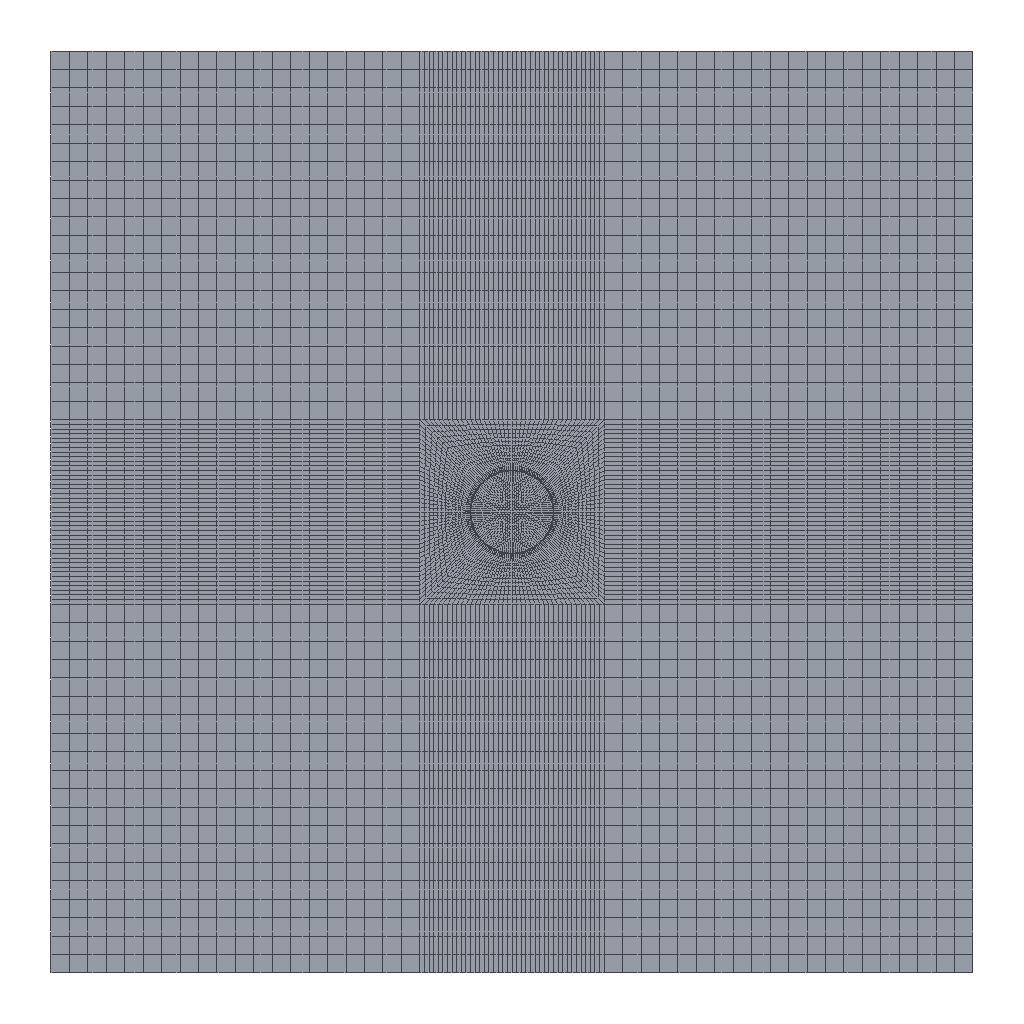Simulation study | abaqus
Set-up summary:
category,name,step,type,value,unit,region
solver,abaqus,,Abaqus/CAE 2024
units,SI m-kg-s (Pa),,inferred,E=2e+10 density=2500
analysis,Step-Geostatic,,geostatic,nlgeom=True; time_period=1
analysis,Step-Excavation,,static,nlgeom=True; time_period=1
analysis,Step-Support,,static,nlgeom=True; time_period=1
analysis,Step-Pressure,,static,nlgeom=True; time_period=8
mesh,nodes,,,10837
mesh,elements,,,10120
element_type,CPE4R,,,8911
element_type,CPE4RH,,,1209
material,Rock,,E,2e+10
material,Rock,,nu,0.25
material,Rock,,density,2500
material,Rubber,,behaviors,hyperelastic
material,UHPC,,E,4.5e+10
material,UHPC,,nu,0.2
material,UHPC,,density,2500
material,UHPC,,behaviors,plastic; concrete damaged plasticity; concrete compression hardening; concrete tension stiffening; concrete compression damage; concrete tension damage
section,Rock,,solid section,,,_PickedSet80
section,Rubber,,solid section,,,_PickedSet2
section,UHPC,,solid section,,,_PickedSet5
load,Load-1,Step-Geostatic,gravity,9.81,,whole model
load,Load-2,Step-Geostatic,pressure,1e+07,,_PickedSurf7
load,Load-3,Step-Geostatic,pressure,1.25e+07,,_PickedSurf8
load,Gas,Step-Pressure,pressure,5e+06,,"Rubber-1.""Rubber inside"""
bc,Bottom,initial,fixed,[dofs=y],,_PickedSet6
bc,Left,initial,fixed,[dofs=x],,_PickedSet4
bc,Right,initial,fixed,[dofs=x],,_PickedSet5
contact,UHPC Rock,initial,tie,,,"UHPC-1.""UHPC outside"" / Cavern-Geostress-1.""Rock inside"""
contact,Int-8,initial,contact pair surface to surface,interaction=Basic 1; friction=0.3; behavior=hard,,"Rubber-1.""Rubber outside"" / UHPC-1.""UHPC inside"""
Abaqus input file, long lists of numbers shortened:
*Heading
** Job name: deck Model name: Model-2
** Generated by: Abaqus/CAE 2024
*Preprint, echo=NO, model=NO, history=NO, contact=NO
**
** PARTS
**
*Part, name=Cavern-Geostress
*Node
      1,         -10.,          10.
      2,         -10.,          50.
** (7999 more lines like these left out)
*Element, type=CPE4R
  1,    1,   30,  970,  105
  2,   30,   31,  971,  970
** (7838 more lines like these left out)
*Nset, nset=_PickedSet80, internal, generate
    1,  8001,     1
*Elset, elset=_PickedSet80, internal, generate
    1,  7840,     1
*Elset, elset="_Rock inside_S2", internal
 2101, 2102, 2103, 2104, 2105, 2106, 2107, 2108, 2109, 2110, 2221, 2222, 2223, 2224, 2225, 2226
 2227, 2228, 2229, 2230, 2341, 2342, 2343, 2344, 2345, 2346, 2347, 2348, 2349, 2350, 2981, 2982
** (3 more lines like these left out)
*Elset, elset="_Rock inside_S1", internal
 2111, 2112, 2113, 2114, 2115, 2116, 2117, 2118, 2119, 2120, 2231, 2232, 2233, 2234, 2235, 2236
 2237, 2238, 2239, 2240, 2351, 2352, 2353, 2354, 2355, 2356, 2357, 2358, 2359, 2360, 2991, 2992
** (3 more lines like these left out)
*Surface, type=ELEMENT, name="Rock inside"
"_Rock inside_S2", S2
"_Rock inside_S1", S1
** Section: Section-1
*Solid Section, elset=_PickedSet80, material=Rock
,
*End Part
**
*Part, name=Rubber
*Node
      1, 0.002345,  -4.5
      2, 0.002345,  -4.46
** (1610 more lines like these left out)
*Element, type=CPE4RH
  1,   1,  18, 823, 121
  2,  18,  19, 824, 823
** (1207 more lines like these left out)
*Nset, nset=_PickedSet2, internal, generate
    1,  1612,     1
*Elset, elset=_PickedSet2, internal, generate
    1,  1209,     1
*Nset, nset="Edge Seeds-Rubber"
   1,   2,   3,   4,   5,   6,   7,   8,   9,  10,  12,  13,  14,  15,  16,  17
  18,  19,  70,  71, 171, 172, 222, 223, 322, 323, 473, 474, 574, 575, 625, 626
*Elset, elset="Edge Seeds-Rubber"
    1,    2,    3,  151,  152,  153,  154,  155,  156,  301,  302,  303,  304,  305,  306,  451
  452,  453,  454,  455,  456,  604,  605,  606,  607,  608,  609,  757,  758,  759,  760,  761
** (1 more lines like these left out)
*Elset, elset="_Rubber outside_S4", internal
    1,    4,    7,   10,   13,   16,   19,   22,   25,   28,   31,   34,   37,   40,   43,   46
   49,   52,   55,   58,   61,   64,   67,   70,   73,   76,   79,   82,   85,   88,   91,   94
** (11 more lines like these left out)
*Elset, elset="_Rubber outside_S2", internal
  156,  159,  162,  165,  168,  171,  174,  177,  180,  183,  186,  189,  192,  195,  198,  201
  204,  207,  210,  213,  216,  219,  222,  225,  228,  231,  234,  237,  240,  243,  246,  249
** (11 more lines like these left out)
*Surface, type=ELEMENT, name="Rubber outside"
"_Rubber outside_S4", S4
"_Rubber outside_S2", S2
*Elset, elset="_Rubber inside_S2", internal
    3,    6,    9,   12,   15,   18,   21,   24,   27,   30,   33,   36,   39,   42,   45,   48
   51,   54,   57,   60,   63,   66,   69,   72,   75,   78,   81,   84,   87,   90,   93,   96
** (11 more lines like these left out)
*Elset, elset="_Rubber inside_S4", internal
  154,  157,  160,  163,  166,  169,  172,  175,  178,  181,  184,  187,  190,  193,  196,  199
  202,  205,  208,  211,  214,  217,  220,  223,  226,  229,  232,  235,  238,  241,  244,  247
** (11 more lines like these left out)
*Surface, type=ELEMENT, name="Rubber inside"
"_Rubber inside_S2", S2
"_Rubber inside_S4", S4
** Section: Section-3
*Solid Section, elset=_PickedSet2, material=Rubber
,
*End Part
**
*Part, name=UHPC
*Node
      1,  -3.536,  -3.536
      2,  -3.182,  -3.182
** (1222 more lines like these left out)
*Element, type=CPE4R
  1,   1,  19, 355,  66
  2,  19,  20, 356, 355
** (1069 more lines like these left out)
*Nset, nset=_PickedSet5, internal, generate
    1,  1224,     1
*Elset, elset=_PickedSet5, internal, generate
    1,  1071,     1
*Elset, elset="_UHPC outside_S4", internal
    1,    8,   15,   22,   29,   36,   43,   50,   57,   64,   71,   78,   85,   92,   99,  106
  113,  120,  127,  400,  407,  414,  421,  428,  435,  442,  449,  456,  463,  470,  477,  484
** (3 more lines like these left out)
*Elset, elset="_UHPC outside_S2", internal
 140, 147, 154, 161, 168, 175, 182, 189, 196, 203, 210, 217, 224, 231, 238, 245
 252, 259, 266, 273, 280, 287, 294, 301, 308, 315, 322, 329, 336, 343, 350, 357
** (3 more lines like these left out)
*Surface, type=ELEMENT, name="UHPC outside"
"_UHPC outside_S4", S4
"_UHPC outside_S2", S2
*Elset, elset="_UHPC inside_S2", internal
    7,   14,   21,   28,   35,   42,   49,   56,   63,   70,   77,   84,   91,   98,  105,  112
  119,  126,  133,  406,  413,  420,  427,  434,  441,  448,  455,  462,  469,  476,  483,  490
** (3 more lines like these left out)
*Elset, elset="_UHPC inside_S4", internal
 134, 141, 148, 155, 162, 169, 176, 183, 190, 197, 204, 211, 218, 225, 232, 239
 246, 253, 260, 267, 274, 281, 288, 295, 302, 309, 316, 323, 330, 337, 344, 351
** (3 more lines like these left out)
*Surface, type=ELEMENT, name="UHPC inside"
"_UHPC inside_S2", S2
"_UHPC inside_S4", S4
** Section: Section-2
*Solid Section, elset=_PickedSet5, material=UHPC
,
*End Part
**
**
** ASSEMBLY
**
*Assembly, name=Assembly
**
*Instance, name=Cavern-Geostress-1, part=Cavern-Geostress
*End Instance
**
*Instance, name=Rubber-1, part=Rubber
*End Instance
**
*Instance, name=UHPC-1, part=UHPC
          0.,           0.,           0.
          0.,           0.,           0.,           0.,           0., 1., 90.
*End Instance
**
*Nset, nset=_PickedSet4, internal, instance=Cavern-Geostress-1
   3,   4,  10,  11,  68,  69,  70,  71,  72,  73,  74,  75,  76,  77,  78,  79
  80,  81,  82,  83,  84,  85,  86, 240, 241, 242, 243, 244, 245, 246, 247, 248
** (4 more lines like these left out)
*Elset, elset=_PickedSet4, internal, instance=Cavern-Geostress-1
  381,  382,  383,  384,  385,  386,  387,  388,  389,  390,  391,  392,  393,  394,  395,  396
  397,  398,  399,  400, 1581, 1582, 1583, 1584, 1585, 1586, 1587, 1588, 1589, 1590, 1591, 1592
** (3 more lines like these left out)
*Nset, nset=_PickedSet5, internal, instance=Cavern-Geostress-1
  14,  15,  25,  29, 316, 317, 318, 319, 320, 321, 322, 323, 324, 325, 326, 327
 328, 329, 330, 331, 332, 333, 334, 653, 654, 655, 656, 657, 658, 659, 660, 661
** (4 more lines like these left out)
*Elset, elset=_PickedSet5, internal, instance=Cavern-Geostress-1
 1981, 1982, 1983, 1984, 1985, 1986, 1987, 1988, 1989, 1990, 1991, 1992, 1993, 1994, 1995, 1996
 1997, 1998, 1999, 2000, 4200, 4220, 4240, 4260, 4280, 4300, 4320, 4340, 4360, 4380, 4400, 4420
** (3 more lines like these left out)
*Nset, nset=_PickedSet6, internal, instance=Cavern-Geostress-1
   8,  11,  13,  14, 259, 260, 261, 262, 263, 264, 265, 266, 267, 268, 269, 270
 271, 272, 273, 274, 275, 276, 277, 297, 298, 299, 300, 301, 302, 303, 304, 305
** (4 more lines like these left out)
*Elset, elset=_PickedSet6, internal, instance=Cavern-Geostress-1
 1201, 1221, 1241, 1261, 1281, 1301, 1321, 1341, 1361, 1381, 1401, 1421, 1441, 1461, 1481, 1501
 1521, 1541, 1561, 1581, 1620, 1640, 1660, 1680, 1700, 1720, 1740, 1760, 1780, 1800, 1820, 1840
** (3 more lines like these left out)
*Nset, nset=_PickedSet10, internal, instance=Cavern-Geostress-1
   16,   17,   18,   19,   20,   23,   24,   26,   27,  354,  355,  356,  357,  358,  359,  360
  361,  362,  363,  364,  365,  366,  367,  368,  369,  370,  371,  372,  373,  374,  375,  376
** (64 more lines like these left out)
*Elset, elset=_PickedSet10, internal, instance=Cavern-Geostress-1
 2001, 2002, 2003, 2004, 2005, 2006, 2007, 2008, 2009, 2010, 2011, 2012, 2013, 2014, 2015, 2016
 2017, 2018, 2019, 2020, 2021, 2022, 2023, 2024, 2025, 2026, 2027, 2028, 2029, 2030, 2031, 2032
** (58 more lines like these left out)
*Nset, nset=_PickedSet32, internal, instance=UHPC-1, generate
    1,  1224,     1
*Elset, elset=_PickedSet32, internal, instance=UHPC-1, generate
    1,  1071,     1
*Nset, nset=_PickedSet33, internal, instance=UHPC-1, generate
    1,  1224,     1
*Elset, elset=_PickedSet33, internal, instance=UHPC-1, generate
    1,  1071,     1
*Nset, nset=_PickedSet34, internal, instance=Rubber-1, generate
    1,  1612,     1
*Elset, elset=_PickedSet34, internal, instance=Rubber-1, generate
    1,  1209,     1
*Nset, nset=_PickedSet35, internal, instance=Rubber-1, generate
    1,  1612,     1
*Elset, elset=_PickedSet35, internal, instance=Rubber-1, generate
    1,  1209,     1
*Elset, elset=__PickedSurf7_S3, internal, instance=Cavern-Geostress-1
  381,  382,  383,  384,  385,  386,  387,  388,  389,  390,  391,  392,  393,  394,  395,  396
  397,  398,  399,  400, 1581, 1582, 1583, 1584, 1585, 1586, 1587, 1588, 1589, 1590, 1591, 1592
** (3 more lines like these left out)
*Elset, elset=__PickedSurf7_S4, internal, instance=Cavern-Geostress-1, generate
 5741,  6521,    20
*Elset, elset=__PickedSurf7_S2, internal, instance=Cavern-Geostress-1, generate
 4200,  4980,    20
*Surface, type=ELEMENT, name=_PickedSurf7, internal
__PickedSurf7_S3, S3
__PickedSurf7_S4, S4
__PickedSurf7_S2, S2
*Elset, elset=__PickedSurf8_S2, internal, instance=Cavern-Geostress-1, generate
   20,  1200,    20
*Elset, elset=__PickedSurf8_S4, internal, instance=Cavern-Geostress-1, generate
 6541,  6921,    20
*Surface, type=ELEMENT, name=_PickedSurf8, internal
__PickedSurf8_S2, S2
__PickedSurf8_S4, S4
** Constraint: UHPC Rock
*Tie, name="UHPC Rock", adjust=yes
UHPC-1."UHPC outside", Cavern-Geostress-1."Rock inside"
*End Assembly
*Amplitude, name=Cycle
             0.,              0.,             0.1,             0.5,             0.2,              1.,              2.,              1.
             3.,             0.8,              4.,             0.5,              5.,             0.2,              6.,              0.
             8.,              0.
**
** MATERIALS
**
*Material, name=Rock
*Density
2500.,
*Elastic
 2e+10, 0.25
*Material, name=Rubber
*Hyperelastic, mooney-rivlin
400000.,100000.,   0.01
*Material, name=UHPC
*Density
2500.,
*Elastic
 4.5e+10, 0.2
*Concrete Damaged Plasticity
30.,    0.1,   1.16, 0.6667,   0.05
*Concrete Compression Hardening
    6e+07,      0.
    7e+07,   5e-05
    8e+07, 0.00012
    9e+07, 0.00022
    1e+08, 0.00036
 1.08e+08, 0.00055
 1.14e+08, 0.00078
 1.19e+08, 0.00105
 1.23e+08, 0.00135
 1.26e+08,  0.0017
 1.25e+08, 0.00205
 1.23e+08, 0.00245
 1.21e+08,  0.0029
 1.18e+08,  0.0034
 1.15e+08,   0.004
 1.11e+08,  0.0047
 1.07e+08,  0.0056
 1.02e+08,  0.0067
  9.6e+07,   0.008
    9e+07,  0.0095
  8.2e+07,  0.0115
  7.4e+07,   0.014
  6.6e+07,   0.017
  5.8e+07,    0.02
*Concrete Tension Stiffening
    1e+07,      0.
 1.15e+07,   2e-05
 1.25e+07,   5e-05
  1.2e+07,  0.0001
  1.1e+07,  0.0002
    1e+07, 0.00035
  8.8e+06, 0.00055
  7.5e+06,  0.0008
  6.2e+06,  0.0012
    5e+06,  0.0018
  3.8e+06,  0.0026
  2.8e+06,  0.0037
    2e+06,  0.0052
  1.2e+06,   0.007
  500000.,    0.01
*Concrete Compression Damage
    0.,      0.
 0.002,   5e-05
 0.005, 0.00012
  0.01, 0.00022
 0.018, 0.00036
  0.03, 0.00055
 0.045, 0.00078
 0.065, 0.00105
  0.09, 0.00135
  0.12,  0.0017
  0.16, 0.00205
  0.21, 0.00245
  0.27,  0.0029
  0.34,  0.0034
  0.42,   0.004
   0.5,  0.0047
  0.58,  0.0056
   0.6,  0.0067
  0.62,   0.008
  0.64,  0.0095
  0.66,  0.0115
  0.68,   0.014
   0.7,   0.017
  0.72,    0.02
*Concrete Tension Damage
   0.,      0.
 0.01,   2e-05
 0.03,   5e-05
 0.06,  0.0001
  0.1,  0.0002
 0.16, 0.00035
 0.24, 0.00055
 0.34,  0.0008
 0.46,  0.0012
 0.58,  0.0018
  0.7,  0.0026
  0.8,  0.0037
 0.88,  0.0052
 0.94,   0.007
 0.99,    0.01
**
** INTERACTION PROPERTIES
**
*Surface Interaction, name="Basic 1"
1.,
*Friction, slip tolerance=0.005
 0.3,
*Surface Behavior, pressure-overclosure=HARD
*Surface Interaction, name="Basic 2"
1.,
*Friction, slip tolerance=0.005
 0.4,
*Surface Behavior, pressure-overclosure=HARD
**
** BOUNDARY CONDITIONS
**
** Name: Bottom bd Type: Displacement/Rotation
*Boundary
_PickedSet6, 2, 2
** Name: Left bd Type: Displacement/Rotation
*Boundary
_PickedSet4, 1, 1
** Name: Right bd Type: Displacement/Rotation
*Boundary
_PickedSet5, 1, 1
**
** INTERACTIONS
**
** Interaction: Int-8
*Contact Pair, interaction="Basic 1", type=SURFACE TO SURFACE
Rubber-1."Rubber outside", UHPC-1."UHPC inside"
** ----------------------------------------------------------------
**
** STEP: Step-Geostatic
**
*Step, name=Step-Geostatic, nlgeom=YES
*Geostatic, utol
0.1, 1., 1e-05, 1.
**
** LOADS
**
** Name: Load-1   Type: Gravity
*Dload
, GRAV, 9.81, 0., -1.
** Name: Load-2   Type: Pressure
*Dsload
_PickedSurf7, P, 1e+07
** Name: Load-3   Type: Pressure
*Dsload
_PickedSurf8, P, 1.25e+07
**
** INTERACTIONS
**
** Interaction: Delete Rubber
*Model Change, remove
_PickedSet34,
** Interaction: Delete UHPC
*Model Change, remove
_PickedSet33,
** Interaction: Int-8
*Model Change, type=CONTACT PAIR, remove
Rubber-1."Rubber outside", UHPC-1."UHPC inside"
**
** OUTPUT REQUESTS
**
*Restart, write, frequency=0
**
** FIELD OUTPUT: F-Output-1
**
*Output, field, variable=PRESELECT
**
** HISTORY OUTPUT: H-Output-1
**
*Output, history, variable=PRESELECT
*End Step
** ----------------------------------------------------------------
**
** STEP: Step-Excavation
**
*Step, name=Step-Excavation, nlgeom=YES, inc=500
*Static, stabilize=0.0002, allsdtol=0.05, continue=NO
0.02, 1., 1e-06, 0.1
**
** INTERACTIONS
**
** Interaction: Delete Rubber
*Model Change, add
_PickedSet34,
** Interaction: Delete UHPC
*Model Change, add
_PickedSet33,
** Interaction: Excavation
*Model Change, remove
_PickedSet10,
** Interaction: Int-8
*Model Change, type=CONTACT PAIR, add
Rubber-1."Rubber outside", UHPC-1."UHPC inside"
**
** OUTPUT REQUESTS
**
*Restart, write, frequency=0
**
** FIELD OUTPUT: F-Output-1
**
*Output, field, variable=PRESELECT
**
** HISTORY OUTPUT: H-Output-1
**
*Output, history, variable=PRESELECT
*End Step
** ----------------------------------------------------------------
**
** STEP: Step-Support
**
*Step, name=Step-Support, nlgeom=YES
Add UHPC Rubber
*Static, stabilize=0.0002, allsdtol=0.05, continue=NO
0.01, 1., 1e-10, 0.1
**
** OUTPUT REQUESTS
**
*Restart, write, frequency=0
**
** FIELD OUTPUT: F-Output-1
**
*Output, field
*Node Output
CF, RF, U
*Element Output, directions=YES
DAMAGEC, DAMAGET, LE, PE, PEEQ, PEMAG, S
*Contact Output
CDISP, CSTRESS
**
** HISTORY OUTPUT: H-Output-1
**
*Output, history, variable=PRESELECT
*End Step
** ----------------------------------------------------------------
**
** STEP: Step-Pressure
**
*Step, name=Step-Pressure, nlgeom=YES, inc=1000
*Static, stabilize=0.0002, allsdtol=0.05, continue=NO
0.001, 8., 1e-10, 0.01
**
** LOADS
**
** Name: Gas Pressure   Type: Pressure
*Dsload, amplitude=Cycle
Rubber-1."Rubber inside", P, 5e+06
**
** OUTPUT REQUESTS
**
*Restart, write, frequency=0
**
** FIELD OUTPUT: F-Output-1
**
*Output, field
*Node Output
CF, RF, U
*Element Output, directions=YES
DAMAGEC, DAMAGET, LE, PE, PEEQ, PEMAG, S
*Contact Output
CDISP, CSTRESS
**
** HISTORY OUTPUT: H-Output-1
**
*Output, history, variable=PRESELECT
*End Step
Results summary:
result,odb.job_status,,,JOB_STATUS_COMPLETED_SUCCESSFULLY,"consistent, unstated (Abaqus has no unit system)"
result,steps[0].procedure,Step-Geostatic,,*GEOSTATIC,"consistent, unstated (Abaqus has no unit system)"
result,steps[0].time_period,Step-Geostatic,,1,"consistent, unstated (Abaqus has no unit system)"
result,steps[0].n_frames,Step-Geostatic,,7,"consistent, unstated (Abaqus has no unit system)"
result,steps[0].last_frame.id,Step-Geostatic,,6,"consistent, unstated (Abaqus has no unit system)"
result,steps[0].last_frame.value,Step-Geostatic,,1,"consistent, unstated (Abaqus has no unit system)"
result,steps[0].last_frame.description,Step-Geostatic,,Increment      6: Step Time =    1.000,"consistent, unstated (Abaqus has no unit system)"
result,steps[0].completed,Step-Geostatic,,True,"consistent, unstated (Abaqus has no unit system)"
result,steps[0].max_U_magnitude,Step-Geostatic,,1.25548e-07,"consistent, unstated (Abaqus has no unit system)"
result,steps[0].max_S_mises,Step-Geostatic,,9.95198e+06,"consistent, unstated (Abaqus has no unit system)"
result,steps[0].RF_sum[1],Step-Geostatic,,26,"consistent, unstated (Abaqus has no unit system)"
result,steps[0].RF_sum[2],Step-Geostatic,,1.49525e+09,"consistent, unstated (Abaqus has no unit system)"
result,steps[1].procedure,Step-Excavation,,*STATIC,"consistent, unstated (Abaqus has no unit system)"
result,steps[1].time_period,Step-Excavation,,1,"consistent, unstated (Abaqus has no unit system)"
result,steps[1].n_frames,Step-Excavation,,15,"consistent, unstated (Abaqus has no unit system)"
result,steps[1].last_frame.id,Step-Excavation,,14,"consistent, unstated (Abaqus has no unit system)"
result,steps[1].last_frame.value,Step-Excavation,,1,"consistent, unstated (Abaqus has no unit system)"
result,steps[1].last_frame.description,Step-Excavation,,Increment     14: Step Time =    1.000,"consistent, unstated (Abaqus has no unit system)"
result,steps[1].completed,Step-Excavation,,True,"consistent, unstated (Abaqus has no unit system)"
result,steps[1].max_U_magnitude,Step-Excavation,,0.00606,"consistent, unstated (Abaqus has no unit system)"
result,steps[1].max_S_mises,Step-Excavation,,4.03912e+07,"consistent, unstated (Abaqus has no unit system)"
result,steps[1].RF_sum[1],Step-Excavation,,77,"consistent, unstated (Abaqus has no unit system)"
result,steps[1].RF_sum[2],Step-Excavation,,1.49367e+09,"consistent, unstated (Abaqus has no unit system)"
result,steps[2].procedure,Step-Support,,*STATIC,"consistent, unstated (Abaqus has no unit system)"
result,steps[2].time_period,Step-Support,,1,"consistent, unstated (Abaqus has no unit system)"
result,steps[2].n_frames,Step-Support,,16,"consistent, unstated (Abaqus has no unit system)"
result,steps[2].last_frame.id,Step-Support,,15,"consistent, unstated (Abaqus has no unit system)"
result,steps[2].last_frame.value,Step-Support,,1,"consistent, unstated (Abaqus has no unit system)"
result,steps[2].last_frame.description,Step-Support,,Increment     15: Step Time =    1.000,"consistent, unstated (Abaqus has no unit system)"
result,steps[2].completed,Step-Support,,True,"consistent, unstated (Abaqus has no unit system)"
result,steps[2].max_U_magnitude,Step-Support,,0.006061,"consistent, unstated (Abaqus has no unit system)"
result,steps[2].max_S_mises,Step-Support,,4.03922e+07,"consistent, unstated (Abaqus has no unit system)"
result,steps[2].RF_sum[1],Step-Support,,87,"consistent, unstated (Abaqus has no unit system)"
result,steps[2].RF_sum[2],Step-Support,,1.49369e+09,"consistent, unstated (Abaqus has no unit system)"
result,steps[3].procedure,Step-Pressure,,*STATIC,"consistent, unstated (Abaqus has no unit system)"
result,steps[3].time_period,Step-Pressure,,8,"consistent, unstated (Abaqus has no unit system)"
result,steps[3].n_frames,Step-Pressure,,810,"consistent, unstated (Abaqus has no unit system)"
result,steps[3].last_frame.id,Step-Pressure,,809,"consistent, unstated (Abaqus has no unit system)"
result,steps[3].last_frame.value,Step-Pressure,,8,"consistent, unstated (Abaqus has no unit system)"
result,steps[3].last_frame.description,Step-Pressure,,Increment    809: Step Time =    8.000,"consistent, unstated (Abaqus has no unit system)"
result,steps[3].completed,Step-Pressure,,True,"consistent, unstated (Abaqus has no unit system)"
result,steps[3].max_U_magnitude,Step-Pressure,,0.006061,"consistent, unstated (Abaqus has no unit system)"
result,steps[3].max_S_mises,Step-Pressure,,4.03922e+07,"consistent, unstated (Abaqus has no unit system)"
result,steps[3].RF_sum[1],Step-Pressure,,55,"consistent, unstated (Abaqus has no unit system)"
result,steps[3].RF_sum[2],Step-Pressure,,1.49369e+09,"consistent, unstated (Abaqus has no unit system)"